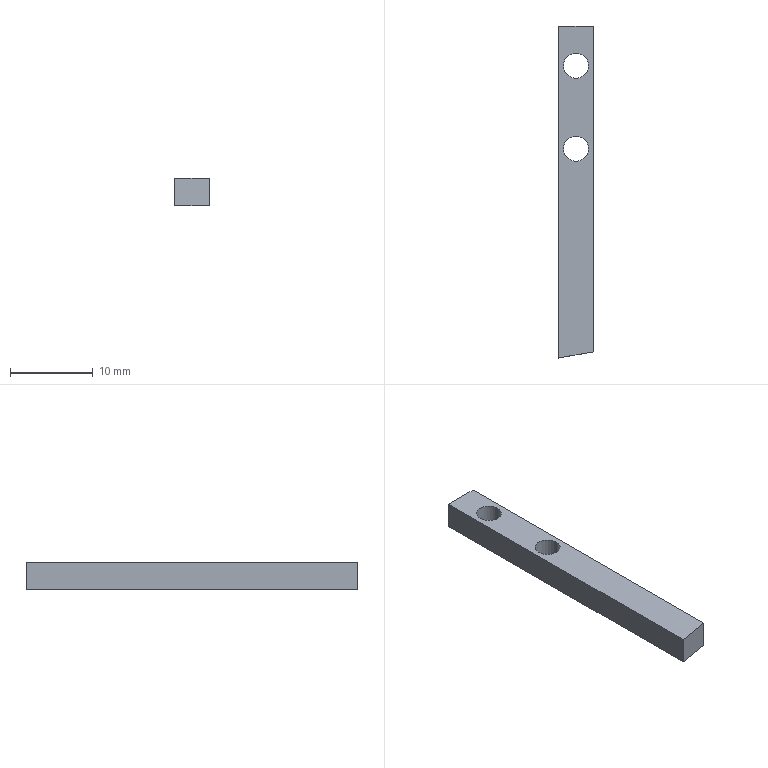Part | SolidWorks | features ICE 2, Extrusion 1 | 1 solid | 10 faces | box 4.18 x 40 x 3.28 mm | volume 496.993 mm3 | plane 6 | cylinder 4 | commonest cylinder face diameters 3 x4
STEP:
#1=CARTESIAN_POINT('',(1.5,25.211,1.64));
#2=VERTEX_POINT('',#1);
#3=CARTESIAN_POINT('',(-1.5,25.211,1.64));
#4=VERTEX_POINT('',#3);
#5=CARTESIAN_POINT('',(0.,25.211,1.64));
#6=DIRECTION('',(0.,0.,-1.));
#7=DIRECTION('',(-1.,0.,0.));
#8=AXIS2_PLACEMENT_3D('',#5,#6,#7);
#9=CIRCLE('',#8,1.5);
#10=EDGE_CURVE('',#2,#4,#9,.T.);
#11=ORIENTED_EDGE('',*,*,#10,.F.);
#12=CARTESIAN_POINT('',(1.5,25.211,-1.64));
#13=VERTEX_POINT('',#12);
#14=CARTESIAN_POINT('',(1.5,25.211,38.36));
#15=DIRECTION('',(0.,0.,-1.));
#16=VECTOR('',#15,1000.);
#17=LINE('',#14,#16);
#18=EDGE_CURVE('',#2,#13,#17,.T.);
#19=ORIENTED_EDGE('',*,*,#18,.T.);
#20=CARTESIAN_POINT('',(-1.5,25.211,-1.64));
#21=VERTEX_POINT('',#20);
#22=CARTESIAN_POINT('',(0.,25.211,-1.64));
#23=DIRECTION('',(0.,0.,-1.));
#24=DIRECTION('',(-1.,0.,0.));
#25=AXIS2_PLACEMENT_3D('',#22,#23,#24);
#26=CIRCLE('',#25,1.5);
#27=EDGE_CURVE('',#13,#21,#26,.T.);
#28=ORIENTED_EDGE('',*,*,#27,.T.);
#29=CARTESIAN_POINT('',(-1.5,25.211,38.36));
#30=DIRECTION('',(0.,0.,-1.));
#31=VECTOR('',#30,1000.);
#32=LINE('',#29,#31);
#33=EDGE_CURVE('',#4,#21,#32,.T.);
#34=ORIENTED_EDGE('',*,*,#33,.F.);
#35=EDGE_LOOP('',(#11,#19,#28,#34));
#36=FACE_OUTER_BOUND('',#35,.T.);
#37=CARTESIAN_POINT('',(0.,25.211,38.36));
#38=DIRECTION('',(0.,0.,-1.));
#39=DIRECTION('',(-1.,0.,0.));
#40=AXIS2_PLACEMENT_3D('',#37,#38,#39);
#41=CYLINDRICAL_SURFACE('',#40,1.5);
#42=ADVANCED_FACE('',(#36),#41,.F.);
#43=CARTESIAN_POINT('',(1.5,35.211,1.64));
#44=VERTEX_POINT('',#43);
#45=CARTESIAN_POINT('',(-1.5,35.211,1.64));
#46=VERTEX_POINT('',#45);
#47=CARTESIAN_POINT('',(0.,35.211,1.64));
#48=DIRECTION('',(0.,0.,-1.));
#49=DIRECTION('',(-1.,0.,0.));
#50=AXIS2_PLACEMENT_3D('',#47,#48,#49);
#51=CIRCLE('',#50,1.5);
#52=EDGE_CURVE('',#44,#46,#51,.T.);
#53=ORIENTED_EDGE('',*,*,#52,.F.);
#54=CARTESIAN_POINT('',(1.5,35.211,-1.64));
#55=VERTEX_POINT('',#54);
#56=CARTESIAN_POINT('',(1.5,35.211,38.36));
#57=DIRECTION('',(0.,0.,-1.));
#58=VECTOR('',#57,1000.);
#59=LINE('',#56,#58);
#60=EDGE_CURVE('',#44,#55,#59,.T.);
#61=ORIENTED_EDGE('',*,*,#60,.T.);
#62=CARTESIAN_POINT('',(-1.5,35.211,-1.64));
#63=VERTEX_POINT('',#62);
#64=CARTESIAN_POINT('',(0.,35.211,-1.64));
#65=DIRECTION('',(0.,0.,-1.));
#66=DIRECTION('',(-1.,0.,0.));
#67=AXIS2_PLACEMENT_3D('',#64,#65,#66);
#68=CIRCLE('',#67,1.5);
#69=EDGE_CURVE('',#55,#63,#68,.T.);
#70=ORIENTED_EDGE('',*,*,#69,.T.);
#71=CARTESIAN_POINT('',(-1.5,35.211,38.36));
#72=DIRECTION('',(0.,0.,-1.));
#73=VECTOR('',#72,1000.);
#74=LINE('',#71,#73);
#75=EDGE_CURVE('',#46,#63,#74,.T.);
#76=ORIENTED_EDGE('',*,*,#75,.F.);
#77=EDGE_LOOP('',(#53,#61,#70,#76));
#78=FACE_OUTER_BOUND('',#77,.T.);
#79=CARTESIAN_POINT('',(0.,35.211,38.36));
#80=DIRECTION('',(0.,0.,-1.));
#81=DIRECTION('',(-1.,0.,0.));
#82=AXIS2_PLACEMENT_3D('',#79,#80,#81);
#83=CYLINDRICAL_SURFACE('',#82,1.5);
#84=ADVANCED_FACE('',(#78),#83,.F.);
#85=CARTESIAN_POINT('',(0.,25.211,1.64));
#86=DIRECTION('',(0.,0.,-1.));
#87=DIRECTION('',(-1.,0.,0.));
#88=AXIS2_PLACEMENT_3D('',#85,#86,#87);
#89=CIRCLE('',#88,1.5);
#90=EDGE_CURVE('',#4,#2,#89,.T.);
#91=ORIENTED_EDGE('',*,*,#90,.T.);
#92=ORIENTED_EDGE('',*,*,#10,.T.);
#93=EDGE_LOOP('',(#91,#92));
#94=FACE_BOUND('',#93,.T.);
#95=CARTESIAN_POINT('',(0.,35.211,1.64));
#96=DIRECTION('',(0.,0.,-1.));
#97=DIRECTION('',(-1.,0.,0.));
#98=AXIS2_PLACEMENT_3D('',#95,#96,#97);
#99=CIRCLE('',#98,1.5);
#100=EDGE_CURVE('',#46,#44,#99,.T.);
#101=ORIENTED_EDGE('',*,*,#100,.T.);
#102=ORIENTED_EDGE('',*,*,#52,.T.);
#103=EDGE_LOOP('',(#101,#102));
#104=FACE_BOUND('',#103,.T.);
#105=CARTESIAN_POINT('',(-2.09,40.,1.64));
#106=VERTEX_POINT('',#105);
#107=CARTESIAN_POINT('',(-2.09,0.,1.64));
#108=VERTEX_POINT('',#107);
#109=CARTESIAN_POINT('',(-2.09,40.,1.64));
#110=DIRECTION('',(0.,-1.,0.));
#111=VECTOR('',#110,1000.);
#112=LINE('',#109,#111);
#113=EDGE_CURVE('',#106,#108,#112,.T.);
#114=ORIENTED_EDGE('',*,*,#113,.T.);
#115=CARTESIAN_POINT('',(2.09,0.737,1.64));
#116=VERTEX_POINT('',#115);
#117=CARTESIAN_POINT('',(2.09,0.737,1.64));
#118=DIRECTION('',(-0.9848,-0.1736,0.));
#119=VECTOR('',#118,1000.);
#120=LINE('',#117,#119);
#121=EDGE_CURVE('',#116,#108,#120,.T.);
#122=ORIENTED_EDGE('',*,*,#121,.F.);
#123=CARTESIAN_POINT('',(2.09,40.,1.64));
#124=VERTEX_POINT('',#123);
#125=CARTESIAN_POINT('',(2.09,40.,1.64));
#126=DIRECTION('',(0.,-1.,0.));
#127=VECTOR('',#126,1000.);
#128=LINE('',#125,#127);
#129=EDGE_CURVE('',#124,#116,#128,.T.);
#130=ORIENTED_EDGE('',*,*,#129,.F.);
#131=CARTESIAN_POINT('',(-2.09,40.,1.64));
#132=DIRECTION('',(1.,0.,0.));
#133=VECTOR('',#132,1000.);
#134=LINE('',#131,#133);
#135=EDGE_CURVE('',#106,#124,#134,.T.);
#136=ORIENTED_EDGE('',*,*,#135,.F.);
#137=EDGE_LOOP('',(#114,#122,#130,#136));
#138=FACE_OUTER_BOUND('',#137,.T.);
#139=CARTESIAN_POINT('',(-2.09,40.,1.64));
#140=DIRECTION('',(0.,0.,-1.));
#141=DIRECTION('',(-1.,0.,0.));
#142=AXIS2_PLACEMENT_3D('',#139,#140,#141);
#143=PLANE('',#142);
#144=ADVANCED_FACE('',(#94,#104,#138),#143,.F.);
#145=ORIENTED_EDGE('',*,*,#129,.T.);
#146=CARTESIAN_POINT('',(2.09,0.737,-1.64));
#147=VERTEX_POINT('',#146);
#148=CARTESIAN_POINT('',(2.09,0.737,-38.36));
#149=DIRECTION('',(0.,0.,1.));
#150=VECTOR('',#149,1000.);
#151=LINE('',#148,#150);
#152=EDGE_CURVE('',#147,#116,#151,.T.);
#153=ORIENTED_EDGE('',*,*,#152,.F.);
#154=CARTESIAN_POINT('',(2.09,40.,-1.64));
#155=VERTEX_POINT('',#154);
#156=CARTESIAN_POINT('',(2.09,40.,-1.64));
#157=DIRECTION('',(0.,-1.,0.));
#158=VECTOR('',#157,1000.);
#159=LINE('',#156,#158);
#160=EDGE_CURVE('',#155,#147,#159,.T.);
#161=ORIENTED_EDGE('',*,*,#160,.F.);
#162=CARTESIAN_POINT('',(2.09,40.,1.64));
#163=DIRECTION('',(0.,0.,-1.));
#164=VECTOR('',#163,1000.);
#165=LINE('',#162,#164);
#166=EDGE_CURVE('',#124,#155,#165,.T.);
#167=ORIENTED_EDGE('',*,*,#166,.F.);
#168=EDGE_LOOP('',(#145,#153,#161,#167));
#169=FACE_OUTER_BOUND('',#168,.T.);
#170=CARTESIAN_POINT('',(2.09,40.,1.64));
#171=DIRECTION('',(-1.,0.,0.));
#172=DIRECTION('',(0.,0.,1.));
#173=AXIS2_PLACEMENT_3D('',#170,#171,#172);
#174=PLANE('',#173);
#175=ADVANCED_FACE('',(#169),#174,.F.);
#176=CARTESIAN_POINT('',(0.,25.211,-1.64));
#177=DIRECTION('',(0.,0.,-1.));
#178=DIRECTION('',(-1.,0.,0.));
#179=AXIS2_PLACEMENT_3D('',#176,#177,#178);
#180=CIRCLE('',#179,1.5);
#181=EDGE_CURVE('',#21,#13,#180,.T.);
#182=ORIENTED_EDGE('',*,*,#181,.F.);
#183=ORIENTED_EDGE('',*,*,#27,.F.);
#184=EDGE_LOOP('',(#182,#183));
#185=FACE_BOUND('',#184,.T.);
#186=CARTESIAN_POINT('',(0.,35.211,-1.64));
#187=DIRECTION('',(0.,0.,-1.));
#188=DIRECTION('',(-1.,0.,0.));
#189=AXIS2_PLACEMENT_3D('',#186,#187,#188);
#190=CIRCLE('',#189,1.5);
#191=EDGE_CURVE('',#63,#55,#190,.T.);
#192=ORIENTED_EDGE('',*,*,#191,.F.);
#193=ORIENTED_EDGE('',*,*,#69,.F.);
#194=EDGE_LOOP('',(#192,#193));
#195=FACE_BOUND('',#194,.T.);
#196=ORIENTED_EDGE('',*,*,#160,.T.);
#197=CARTESIAN_POINT('',(-2.09,0.,-1.64));
#198=VERTEX_POINT('',#197);
#199=CARTESIAN_POINT('',(8.804,1.921,-1.64));
#200=DIRECTION('',(-0.9848,-0.1736,0.));
#201=VECTOR('',#200,1000.);
#202=LINE('',#199,#201);
#203=EDGE_CURVE('',#147,#198,#202,.T.);
#204=ORIENTED_EDGE('',*,*,#203,.T.);
#205=CARTESIAN_POINT('',(-2.09,40.,-1.64));
#206=VERTEX_POINT('',#205);
#207=CARTESIAN_POINT('',(-2.09,40.,-1.64));
#208=DIRECTION('',(0.,-1.,0.));
#209=VECTOR('',#208,1000.);
#210=LINE('',#207,#209);
#211=EDGE_CURVE('',#206,#198,#210,.T.);
#212=ORIENTED_EDGE('',*,*,#211,.F.);
#213=CARTESIAN_POINT('',(2.09,40.,-1.64));
#214=DIRECTION('',(-1.,0.,0.));
#215=VECTOR('',#214,1000.);
#216=LINE('',#213,#215);
#217=EDGE_CURVE('',#155,#206,#216,.T.);
#218=ORIENTED_EDGE('',*,*,#217,.F.);
#219=EDGE_LOOP('',(#196,#204,#212,#218));
#220=FACE_OUTER_BOUND('',#219,.T.);
#221=CARTESIAN_POINT('',(2.09,40.,-1.64));
#222=DIRECTION('',(0.,0.,1.));
#223=DIRECTION('',(1.,0.,0.));
#224=AXIS2_PLACEMENT_3D('',#221,#222,#223);
#225=PLANE('',#224);
#226=ADVANCED_FACE('',(#185,#195,#220),#225,.F.);
#227=CARTESIAN_POINT('',(-2.09,0.,-1.64));
#228=DIRECTION('',(0.,0.,1.));
#229=VECTOR('',#228,1000.);
#230=LINE('',#227,#229);
#231=EDGE_CURVE('',#198,#108,#230,.T.);
#232=ORIENTED_EDGE('',*,*,#231,.T.);
#233=ORIENTED_EDGE('',*,*,#113,.F.);
#234=CARTESIAN_POINT('',(-2.09,40.,-1.64));
#235=DIRECTION('',(0.,0.,1.));
#236=VECTOR('',#235,1000.);
#237=LINE('',#234,#236);
#238=EDGE_CURVE('',#206,#106,#237,.T.);
#239=ORIENTED_EDGE('',*,*,#238,.F.);
#240=ORIENTED_EDGE('',*,*,#211,.T.);
#241=EDGE_LOOP('',(#232,#233,#239,#240));
#242=FACE_OUTER_BOUND('',#241,.T.);
#243=CARTESIAN_POINT('',(-2.09,40.,-1.64));
#244=DIRECTION('',(1.,0.,0.));
#245=DIRECTION('',(0.,0.,-1.));
#246=AXIS2_PLACEMENT_3D('',#243,#244,#245);
#247=PLANE('',#246);
#248=ADVANCED_FACE('',(#242),#247,.F.);
#249=ORIENTED_EDGE('',*,*,#135,.T.);
#250=ORIENTED_EDGE('',*,*,#166,.T.);
#251=ORIENTED_EDGE('',*,*,#217,.T.);
#252=ORIENTED_EDGE('',*,*,#238,.T.);
#253=EDGE_LOOP('',(#249,#250,#251,#252));
#254=FACE_OUTER_BOUND('',#253,.T.);
#255=CARTESIAN_POINT('',(0.,40.,0.));
#256=DIRECTION('',(0.,1.,0.));
#257=DIRECTION('',(0.,0.,1.));
#258=AXIS2_PLACEMENT_3D('',#255,#256,#257);
#259=PLANE('',#258);
#260=ADVANCED_FACE('',(#254),#259,.T.);
#261=ORIENTED_EDGE('',*,*,#152,.T.);
#262=ORIENTED_EDGE('',*,*,#121,.T.);
#263=ORIENTED_EDGE('',*,*,#231,.F.);
#264=ORIENTED_EDGE('',*,*,#203,.F.);
#265=EDGE_LOOP('',(#261,#262,#263,#264));
#266=FACE_OUTER_BOUND('',#265,.T.);
#267=CARTESIAN_POINT('',(2.09,0.737,-38.36));
#268=DIRECTION('',(-0.1736,0.9848,0.));
#269=DIRECTION('',(-0.9848,-0.1736,0.));
#270=AXIS2_PLACEMENT_3D('',#267,#268,#269);
#271=PLANE('',#270);
#272=ADVANCED_FACE('',(#266),#271,.F.);
#273=ORIENTED_EDGE('',*,*,#60,.F.);
#274=ORIENTED_EDGE('',*,*,#100,.F.);
#275=ORIENTED_EDGE('',*,*,#75,.T.);
#276=ORIENTED_EDGE('',*,*,#191,.T.);
#277=EDGE_LOOP('',(#273,#274,#275,#276));
#278=FACE_OUTER_BOUND('',#277,.T.);
#279=CARTESIAN_POINT('',(0.,35.211,38.36));
#280=DIRECTION('',(0.,0.,-1.));
#281=DIRECTION('',(-1.,0.,0.));
#282=AXIS2_PLACEMENT_3D('',#279,#280,#281);
#283=CYLINDRICAL_SURFACE('',#282,1.5);
#284=ADVANCED_FACE('',(#278),#283,.F.);
#285=ORIENTED_EDGE('',*,*,#18,.F.);
#286=ORIENTED_EDGE('',*,*,#90,.F.);
#287=ORIENTED_EDGE('',*,*,#33,.T.);
#288=ORIENTED_EDGE('',*,*,#181,.T.);
#289=EDGE_LOOP('',(#285,#286,#287,#288));
#290=FACE_OUTER_BOUND('',#289,.T.);
#291=CARTESIAN_POINT('',(0.,25.211,38.36));
#292=DIRECTION('',(0.,0.,-1.));
#293=DIRECTION('',(-1.,0.,0.));
#294=AXIS2_PLACEMENT_3D('',#291,#292,#293);
#295=CYLINDRICAL_SURFACE('',#294,1.5);
#296=ADVANCED_FACE('',(#290),#295,.F.);
#297=CLOSED_SHELL('',(#42,#84,#144,#175,#226,#248,#260,#272,#284,#296));
#298=MANIFOLD_SOLID_BREP('',#297);
#299=CARTESIAN_POINT('',(0.,0.,0.));
#300=DIRECTION('',(0.,0.,1.));
#301=DIRECTION('',(1.,0.,0.));
#302=AXIS2_PLACEMENT_3D('',#299,#300,#301);
#303=(LENGTH_UNIT()NAMED_UNIT(*)SI_UNIT(.MILLI.,.METRE.));
#304=UNCERTAINTY_MEASURE_WITH_UNIT(LENGTH_MEASURE(0.00001),#303,'','');
#305=(NAMED_UNIT(*)PLANE_ANGLE_UNIT()SI_UNIT($,.RADIAN.));
#306=(NAMED_UNIT(*)SI_UNIT($,.STERADIAN.)SOLID_ANGLE_UNIT());
#307=(GEOMETRIC_REPRESENTATION_CONTEXT(3)GLOBAL_UNCERTAINTY_ASSIGNED_CONTEXT((#304))GLOBAL_UNIT_ASSIGNED_CONTEXT((#303,#305,#306))REPRESENTATION_CONTEXT('',''));
#308=ADVANCED_BREP_SHAPE_REPRESENTATION('',(#298,#302),#307);